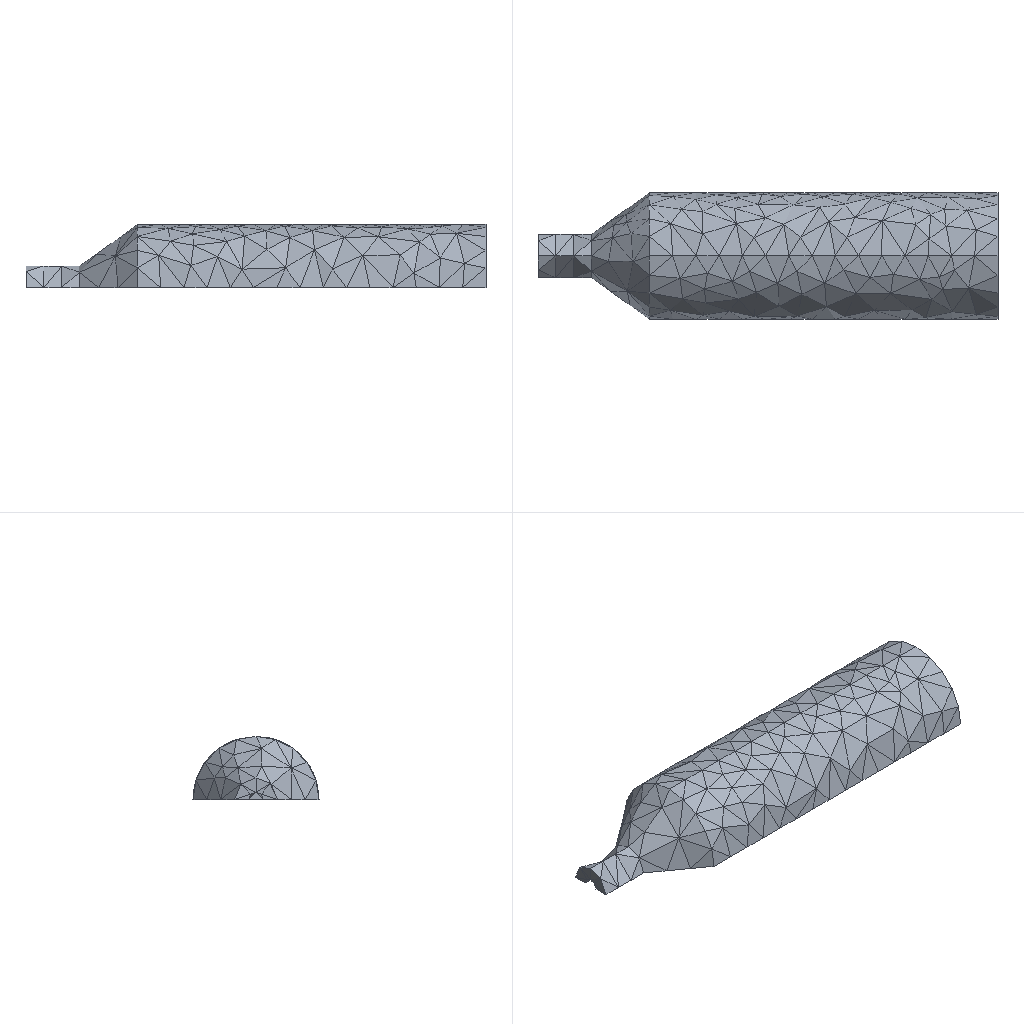Simulation study | ansys workbench
Ansys APDL input file, long lists of numbers shortened:
/batch
/config,noeldb,1     ! force off writing results to database
*get,_wallstrt,active,,time,wall
! ANSYS input file written by Workbench version 2022 R1
! File used for geometry attach:
/title,wbnew--____ (B5)
! ****** Begin Custom Load Command Snippet ******
/COM, ACT Extensions:
/COM,     LSDYNA, 2021.1
/COM,
! ****** End   Custom Load Command Snippet ******
*DIM,_wb_ProjectScratch_dir,string,248
_wb_ProjectScratch_dir(1) = ''
*DIM,_wb_SolverFiles_dir,string,248
_wb_SolverFiles_dir(1) = ''
*DIM,_wb_userfiles_dir,string,248
_wb_userfiles_dir(1) = ''
/com,--- Data in consistent NMM units. See Solving Units in the help system for more information.
/units,MPA
/nopr
/wb,file,start              !  signify a WB generated input file
/prep7
! Turn off shape checking because checks already performed inside WB mesher.
! See help system for more information.
SHPP,OFF,,NOWARN
/nolist
etcon,set             ! allow ANSYS to choose best KEYOP's for 180x elements, resets any applicable keyopt to MAPDL defaults
/com,*********** Nodes for the whole assembly ***********
nblock,3,,1898
(1i9,3e20.9e3)
        1     1.255000000E+03     0.000000000E+00     1.389968367E+02
! (1725 more lines like these left out)
-1
/wb,elem,start            !  set before creation of elements
/com,*********** Elements for Body 1 "__2-FreeParts|__-__2" ***********
et,1,187
eblock,19,solid,,784
(19i9)
        1        1        1        1        0        0        0        0       10        0        1      227      306      247      297     1478     1582     1476     1477
! (1567 more lines like these left out)
-1
/wb,elem,end               !  done creating elements
/com,*********** Send User Defined Coordinate System(s) ***********
csys,0
toffst,273.15,  ! Temperature offset from absolute zero
/com,*********** Set Reference Temperature ***********
tref,22.
/wb,mat,start              !  starting to send materials
/com,*********** Send Materials ***********
Temperature = 'TEMP' ! Temperature
MP,DENS,1,7.85e-09,	! tonne mm^-3
MP,ALPX,1,1.2e-05,	! C^-1
MP,C,1,434000000,	! mm^2 s^-2 C^-1
MP,KXX,1,60.5,	! tonne mm s^-3 C^-1
MP,RSVX,1,0.00017,	! ohm mm
MP,EX,1,200000,	! tonne s^-2 mm^-1
MP,NUXY,1,0.3,
MP,MURX,1,10000,
/wb,mat,end                !  done sending materials
!************************* Model Summary ********************
!__2-FreeParts|__-__2,	结构钢,	matid,	1
!************************* End Model Summary ********************
! get the diagonal of the bounding box. Needed later for other things
*get,_xmin,node,,mnloc,x
*get,_ymin,node,,mnloc,y
*get,_zmin,node,,mnloc,z
*get,_xmax,node,,mxloc,x
*get,_ymax,node,,mxloc,y
*get,_zmax,node,,mxloc,z
_ASMDIAG=(_xmax-_xmin)*(_xmax-_xmin)+(_ymax-_ymin)*(_ymax-_ymin)+(_zmax-_zmin)*(_zmax-_zmin)
_ASMDIAG=SQRT(_ASMDIAG)
/wb,contact,start          !  starting to send contact
/wb,contact,end            !  done creating contacts
/golist
/wb,load,start             !  starting to send loads
/com,*********** Fixed Supports ***********
CMBLOCK,_FIXEDSU,NODE,       49
(8i10)
        57        58        59        60        61        62        97        98
        99       100       101       102       103       104       105       106
       313       733       735       737       739       740       741       743
       747       748       749       754       755       759       763       955
       956       958       963       967       968       971       972       973
       974       977       978       979       981       983       984       987
       988
cmsel,s,_FIXEDSU
d,all,all
nsel,all
/com,*********** Define Pressure Using Surface Effect Elements "__" ***********
et,2,154
eblock,10,,,234
(15i9)
     1411        2        2        2        0       58      103       64       64      739      769       64      738
! (233 more lines like these left out)
-1
esel,s,type,,2
keyop,2,7,0                ! Use deformed area for application of load
esel,all
/com,*********** Define Pressure Using Surface Effect Elements "__ 2" ***********
et,3,154
eblock,10,,,164
(15i9)
     1645        3        3        3        0        8      300      288      288      395     1679      288      394
! (163 more lines like these left out)
-1
esel,s,type,,3
keyop,3,7,0                ! Use deformed area for application of load
esel,all
esel,all
/gst,on,on
fini
*get,_numnode,node,0,count
*get,_numelem,elem,0,count
*get, _MAXELEMNUM, elem, 0, NUM, MAX
*get, _MAXNODENUM, node, 0, NUM, MAX
*get, _MAXELEMTYPE, etyp, 0, NUM, MAX
*get, _MAXREALCONST, real, 0, NUM, MAX
/go
/wb,load,end               !  done creating loads
/com,--- Number of total nodes = %_numnode%
/com,--- Number of contact elements = 398
/com,--- Number of spring elements = 0
/com,--- Number of bearing elements = 0
/com,--- Number of solid elements = 784
/com,--- Number of condensed parts = 0
/com,--- Number of total elements = %_numelem%
*get,_wallbsol,active,,time,wall
/com,****************************************************************************
/com,*************************    SOLUTION       ********************************
/com,****************************************************************************
/solu
antype,0                   ! static analysis
_thickRatio=  0     ! Ratio of thick parts in the model
eqsl,sparse,,,,,1
cntr,print,1               ! print out contact info and also make no initial contact an error
dmpoption,emat,no             ! Don't combine emat file for DANSYS
dmpoption,esav,no             ! Don't combine esav file for DANSYS
nldiag,cont,iter           ! print out contact info each equilibrium iteration
rescontrol,,none                 ! Do not keep any restart files
/com,****************************************************
/com,******************* SOLVE FOR LS 1 OF 1 ****************
esel,s,type,,2
nsle
sf,all,pres,20.
esel,s,type,,3
nsle
sf,all,pres,60.
nsel,all
esel,all
esel,all
/nopr
/gopr
nsub,1,1,1
time,1.
outres,erase
outres,all,none
outres,nsol,all,
outres,rsol,all
outres,eangl,all
outres,etmp,all
outres,veng,all
outres,strs,all,
outres,epel,all,
outres,eppl,all,
outres,cont,all,
! *********** WB SOLVE COMMAND ***********
! check interactive state
*get,ANSINTER_,active,,int
*if,ANSINTER_,ne,0,then
/eof
*endif
solve
/com *************** Write FE CONNECTORS *********
CEWRITE,file,ce,,INTE
/com,****************************************************
/com,*************** FINISHED SOLVE FOR LS 1 *************
*get,_wallasol,active,,time,wall
/nopr
*get,_numnode,node,0,count
*get,_numelem,elem,0,count
*get, _MAXELEMNUM, elem, 0, NUM, MAX
*get, _MAXNODENUM, node, 0, NUM, MAX,,,INTERNAL
*get, _MAXELEMTYPE, etyp, 0, NUM, MAX
*get, _MAXREALCONST, real, 0, NUM, MAX
/gopr
/post1
xmlo,ENCODING,ISO-8859-1
xmlo,parm
/xml,parm,xml
fini
/gopr
*get,_walldone,active,,time,wall
_preptime=(_wallbsol-_wallstrt)*3600
_solvtime=(_wallasol-_wallbsol)*3600
_posttime=(_walldone-_wallasol)*3600
_totaltim=(_walldone-_wallstrt)*3600
*get,_dlbratio,active,0,solu,dlbr
*get,_combtime,active,0,solu,comb
*get,_ssmode,active,0,solu,ssmm
*get,_ndofs,active,0,solu,ndof
*get,_sol_end_time,active,0,set,time
*if,_sol_end_time,eq,1.,then
/fclean				!clean distributed files
*endif
/com,--- Total number of nodes = %_numnode%
/com,--- Total number of elements = %_numelem%
/com,--- Element load balance ratio = %_dlbratio%
/com,--- Time to combine distributed files = %_combtime%
/com,--- Sparse memory mode = %_ssmode%
/com,--- Number of DOF = %_ndofs%
/wb,file,end               ! done with WB generated input